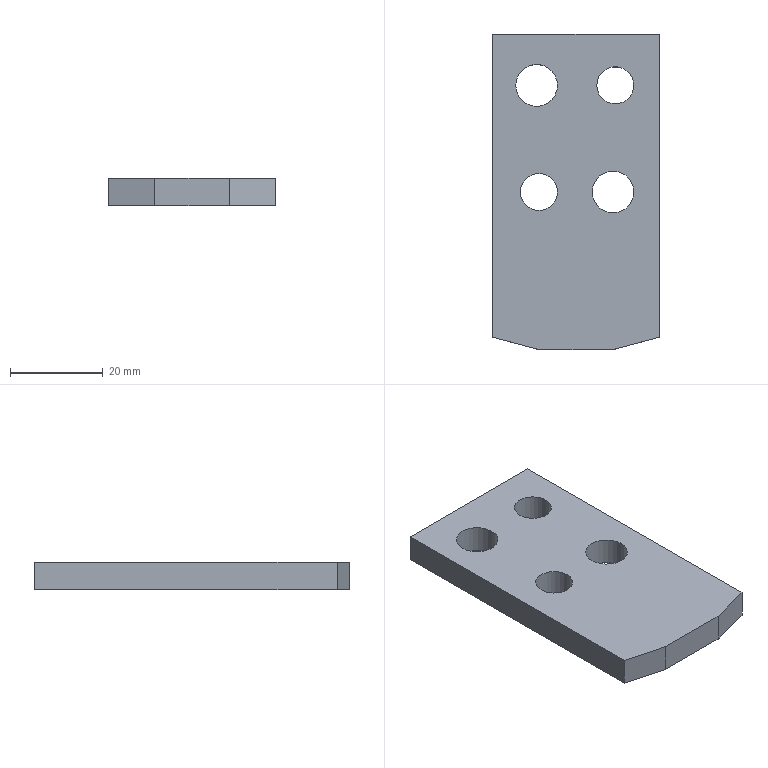Part | STEP file | gslz 2016.10.28-13_id1742_x_t | 1 solid | 12 faces | box 36 x 68 x 6 mm | volume 13161 mm3 | plane 8 | cylinder 4 | commonest cylinder face diameters 8 x2 9 x2
STEP:
#1=CARTESIAN_POINT('',(0.,0.,0.));
#2=DIRECTION('',(0.,0.,1.));
#3=DIRECTION('',(1.,0.,0.));
#4=AXIS2_PLACEMENT_3D('',#1,#2,#3);
#5=CARTESIAN_POINT('',(-870.002,304.2,6.));
#6=VERTEX_POINT('',#5);
#7=CARTESIAN_POINT('',(-878.002,304.2,6.));
#8=VERTEX_POINT('',#7);
#9=CARTESIAN_POINT('',(-874.002,304.2,6.));
#10=DIRECTION('',(0.,0.,1.));
#11=DIRECTION('',(-1.,0.,0.));
#12=AXIS2_PLACEMENT_3D('',#9,#10,#11);
#13=CIRCLE('',#12,4.);
#14=CARTESIAN_POINT('',(-874.002,304.2,-73.));
#15=DIRECTION('',(0.,0.,1.));
#16=DIRECTION('',(1.,0.,0.));
#17=AXIS2_PLACEMENT_3D('',#14,#15,#16);
#18=CYLINDRICAL_SURFACE('',#17,4.);
#19=CARTESIAN_POINT('',(-3.142,79.));
#20=DIRECTION('',(1.,0.));
#21=VECTOR('',#20,1.);
#22=LINE('',#19,#21);
#23=(GEOMETRIC_REPRESENTATION_CONTEXT(2)PARAMETRIC_REPRESENTATION_CONTEXT()REPRESENTATION_CONTEXT('',''));
#24=DEFINITIONAL_REPRESENTATION('',(#22),#23);
#25=PCURVE('',#18,#24);
#26=CARTESIAN_POINT('',(-941.002,267.7,6.));
#27=DIRECTION('',(0.,0.,-1.));
#28=DIRECTION('',(-1.,0.,0.));
#29=AXIS2_PLACEMENT_3D('',#26,#27,#28);
#30=PLANE('',#29);
#31=CARTESIAN_POINT('',(-63.,36.5));
#32=CARTESIAN_POINT('',(-63.,29.572));
#33=CARTESIAN_POINT('',(-69.,33.036));
#34=CARTESIAN_POINT('',(-75.,36.5));
#35=CARTESIAN_POINT('',(-69.,39.964));
#36=CARTESIAN_POINT('',(-63.,43.428));
#37=CARTESIAN_POINT('',(-63.,36.5));
#38=(BOUNDED_CURVE()B_SPLINE_CURVE(2,(#31,#32,#33,#34,#35,#36,#37),.UNSPECIFIED.,.T.,.F.)B_SPLINE_CURVE_WITH_KNOTS((1,2,2,2,2,1),(-2.094,0.,2.094,4.189,6.283,8.378),.UNSPECIFIED.)CURVE()GEOMETRIC_REPRESENTATION_ITEM()RATIONAL_B_SPLINE_CURVE((1.,0.5,1.,0.5,1.,0.5,1.))REPRESENTATION_ITEM(''));
#39=(GEOMETRIC_REPRESENTATION_CONTEXT(2)PARAMETRIC_REPRESENTATION_CONTEXT()REPRESENTATION_CONTEXT('',''));
#40=DEFINITIONAL_REPRESENTATION('',(#38),#39);
#41=PCURVE('',#30,#40);
#42=SURFACE_CURVE('',#13,(#25,#41),.PCURVE_S1.);
#43=EDGE_CURVE('',#6,#8,#42,.T.);
#44=ORIENTED_EDGE('',*,*,#43,.F.);
#45=CARTESIAN_POINT('',(-870.002,304.2,0.));
#46=VERTEX_POINT('',#45);
#47=CARTESIAN_POINT('',(-870.002,304.2,0.));
#48=CARTESIAN_POINT('',(-870.002,304.2,6.));
#49=B_SPLINE_CURVE_WITH_KNOTS('',1,(#47,#48),.UNSPECIFIED.,.F.,.F.,(2,2),(73.,79.),.PIECEWISE_BEZIER_KNOTS.);
#50=CARTESIAN_POINT('',(0.,0.));
#51=DIRECTION('',(0.,1.));
#52=VECTOR('',#51,1.);
#53=LINE('',#50,#52);
#54=(GEOMETRIC_REPRESENTATION_CONTEXT(2)PARAMETRIC_REPRESENTATION_CONTEXT()REPRESENTATION_CONTEXT('',''));
#55=DEFINITIONAL_REPRESENTATION('',(#53),#54);
#56=PCURVE('',#18,#55);
#57=CARTESIAN_POINT('',(6.283,0.));
#58=DIRECTION('',(0.,1.));
#59=VECTOR('',#58,1.);
#60=LINE('',#57,#59);
#61=(GEOMETRIC_REPRESENTATION_CONTEXT(2)PARAMETRIC_REPRESENTATION_CONTEXT()REPRESENTATION_CONTEXT('',''));
#62=DEFINITIONAL_REPRESENTATION('',(#60),#61);
#63=PCURVE('',#18,#62);
#64=SEAM_CURVE('',#49,(#56,#63),.PCURVE_S1.);
#65=EDGE_CURVE('',#46,#6,#64,.T.);
#66=ORIENTED_EDGE('',*,*,#65,.F.);
#67=CARTESIAN_POINT('',(-874.002,304.2,0.));
#68=DIRECTION('',(0.,0.,-1.));
#69=DIRECTION('',(1.,0.,0.));
#70=AXIS2_PLACEMENT_3D('',#67,#68,#69);
#71=CIRCLE('',#70,4.);
#72=CARTESIAN_POINT('',(6.283,73.));
#73=DIRECTION('',(-1.,0.));
#74=VECTOR('',#73,1.);
#75=LINE('',#72,#74);
#76=(GEOMETRIC_REPRESENTATION_CONTEXT(2)PARAMETRIC_REPRESENTATION_CONTEXT()REPRESENTATION_CONTEXT('',''));
#77=DEFINITIONAL_REPRESENTATION('',(#75),#76);
#78=PCURVE('',#18,#77);
#79=CARTESIAN_POINT('',(-981.002,298.2,0.));
#80=DIRECTION('',(0.,0.,1.));
#81=DIRECTION('',(1.,0.,0.));
#82=AXIS2_PLACEMENT_3D('',#79,#80,#81);
#83=PLANE('',#82);
#84=CARTESIAN_POINT('',(111.,6.));
#85=CARTESIAN_POINT('',(111.,-0.9282));
#86=CARTESIAN_POINT('',(105.,2.536));
#87=CARTESIAN_POINT('',(99.,6.));
#88=CARTESIAN_POINT('',(105.,9.464));
#89=CARTESIAN_POINT('',(111.,12.928));
#90=CARTESIAN_POINT('',(111.,6.));
#91=(BOUNDED_CURVE()B_SPLINE_CURVE(2,(#84,#85,#86,#87,#88,#89,#90),.UNSPECIFIED.,.T.,.F.)B_SPLINE_CURVE_WITH_KNOTS((1,2,2,2,2,1),(-2.094,0.,2.094,4.189,6.283,8.378),.UNSPECIFIED.)CURVE()GEOMETRIC_REPRESENTATION_ITEM()RATIONAL_B_SPLINE_CURVE((1.,0.5,1.,0.5,1.,0.5,1.))REPRESENTATION_ITEM(''));
#92=(GEOMETRIC_REPRESENTATION_CONTEXT(2)PARAMETRIC_REPRESENTATION_CONTEXT()REPRESENTATION_CONTEXT('',''));
#93=DEFINITIONAL_REPRESENTATION('',(#91),#92);
#94=PCURVE('',#83,#93);
#95=SURFACE_CURVE('',#71,(#78,#94),.PCURVE_S1.);
#96=EDGE_CURVE('',#46,#46,#95,.T.);
#97=ORIENTED_EDGE('',*,*,#96,.F.);
#98=ORIENTED_EDGE('',*,*,#65,.T.);
#99=CARTESIAN_POINT('',(-874.002,304.2,6.));
#100=DIRECTION('',(0.,0.,1.));
#101=DIRECTION('',(-1.,0.,0.));
#102=AXIS2_PLACEMENT_3D('',#99,#100,#101);
#103=CIRCLE('',#102,4.);
#104=CARTESIAN_POINT('',(3.142,79.));
#105=DIRECTION('',(1.,0.));
#106=VECTOR('',#105,1.);
#107=LINE('',#104,#106);
#108=(GEOMETRIC_REPRESENTATION_CONTEXT(2)PARAMETRIC_REPRESENTATION_CONTEXT()REPRESENTATION_CONTEXT('',''));
#109=DEFINITIONAL_REPRESENTATION('',(#107),#108);
#110=PCURVE('',#18,#109);
#111=CARTESIAN_POINT('',(-63.,36.5));
#112=CARTESIAN_POINT('',(-63.,29.572));
#113=CARTESIAN_POINT('',(-69.,33.036));
#114=CARTESIAN_POINT('',(-75.,36.5));
#115=CARTESIAN_POINT('',(-69.,39.964));
#116=CARTESIAN_POINT('',(-63.,43.428));
#117=CARTESIAN_POINT('',(-63.,36.5));
#118=(BOUNDED_CURVE()B_SPLINE_CURVE(2,(#111,#112,#113,#114,#115,#116,#117),.UNSPECIFIED.,.T.,.F.)B_SPLINE_CURVE_WITH_KNOTS((1,2,2,2,2,1),(-2.094,0.,2.094,4.189,6.283,8.378),.UNSPECIFIED.)CURVE()GEOMETRIC_REPRESENTATION_ITEM()RATIONAL_B_SPLINE_CURVE((1.,0.5,1.,0.5,1.,0.5,1.))REPRESENTATION_ITEM(''));
#119=(GEOMETRIC_REPRESENTATION_CONTEXT(2)PARAMETRIC_REPRESENTATION_CONTEXT()REPRESENTATION_CONTEXT('',''));
#120=DEFINITIONAL_REPRESENTATION('',(#118),#119);
#121=PCURVE('',#30,#120);
#122=SURFACE_CURVE('',#103,(#110,#121),.PCURVE_S1.);
#123=EDGE_CURVE('',#8,#6,#122,.T.);
#124=ORIENTED_EDGE('',*,*,#123,.F.);
#125=EDGE_LOOP('',(#44,#66,#97,#98,#124));
#126=FACE_BOUND('',#125,.F.);
#127=ADVANCED_FACE('',(#126),#18,.F.);
#128=CARTESIAN_POINT('',(-862.502,304.2,6.));
#129=VERTEX_POINT('',#128);
#130=CARTESIAN_POINT('',(-853.502,304.2,6.));
#131=VERTEX_POINT('',#130);
#132=CARTESIAN_POINT('',(-858.002,304.2,6.));
#133=DIRECTION('',(0.,0.,-1.));
#134=DIRECTION('',(-1.,0.,0.));
#135=AXIS2_PLACEMENT_3D('',#132,#133,#134);
#136=CIRCLE('',#135,4.5);
#137=CARTESIAN_POINT('',(-858.002,304.2,-73.));
#138=DIRECTION('',(0.,0.,1.));
#139=DIRECTION('',(1.,0.,0.));
#140=AXIS2_PLACEMENT_3D('',#137,#138,#139);
#141=CYLINDRICAL_SURFACE('',#140,4.5);
#142=CARTESIAN_POINT('',(3.142,79.));
#143=DIRECTION('',(-1.,0.));
#144=VECTOR('',#143,1.);
#145=LINE('',#142,#144);
#146=(GEOMETRIC_REPRESENTATION_CONTEXT(2)PARAMETRIC_REPRESENTATION_CONTEXT()REPRESENTATION_CONTEXT('',''));
#147=DEFINITIONAL_REPRESENTATION('',(#145),#146);
#148=PCURVE('',#141,#147);
#149=CARTESIAN_POINT('',(-83.,36.5));
#150=DIRECTION('',(1.,0.));
#151=AXIS2_PLACEMENT_2D('',#149,#150);
#152=CIRCLE('',#151,4.5);
#153=(GEOMETRIC_REPRESENTATION_CONTEXT(2)PARAMETRIC_REPRESENTATION_CONTEXT()REPRESENTATION_CONTEXT('',''));
#154=DEFINITIONAL_REPRESENTATION('',(#152),#153);
#155=PCURVE('',#30,#154);
#156=SURFACE_CURVE('',#136,(#148,#155),.PCURVE_S1.);
#157=EDGE_CURVE('',#129,#131,#156,.T.);
#158=ORIENTED_EDGE('',*,*,#157,.T.);
#159=CARTESIAN_POINT('',(-853.502,304.2,0.));
#160=VERTEX_POINT('',#159);
#161=CARTESIAN_POINT('',(-853.502,304.2,0.));
#162=CARTESIAN_POINT('',(-853.502,304.2,6.));
#163=B_SPLINE_CURVE_WITH_KNOTS('',1,(#161,#162),.UNSPECIFIED.,.F.,.F.,(2,2),(73.,79.),.PIECEWISE_BEZIER_KNOTS.);
#164=CARTESIAN_POINT('',(0.,0.));
#165=DIRECTION('',(0.,1.));
#166=VECTOR('',#165,1.);
#167=LINE('',#164,#166);
#168=(GEOMETRIC_REPRESENTATION_CONTEXT(2)PARAMETRIC_REPRESENTATION_CONTEXT()REPRESENTATION_CONTEXT('',''));
#169=DEFINITIONAL_REPRESENTATION('',(#167),#168);
#170=PCURVE('',#141,#169);
#171=CARTESIAN_POINT('',(6.283,0.));
#172=DIRECTION('',(0.,1.));
#173=VECTOR('',#172,1.);
#174=LINE('',#171,#173);
#175=(GEOMETRIC_REPRESENTATION_CONTEXT(2)PARAMETRIC_REPRESENTATION_CONTEXT()REPRESENTATION_CONTEXT('',''));
#176=DEFINITIONAL_REPRESENTATION('',(#174),#175);
#177=PCURVE('',#141,#176);
#178=SEAM_CURVE('',#163,(#170,#177),.PCURVE_S1.);
#179=EDGE_CURVE('',#160,#131,#178,.T.);
#180=ORIENTED_EDGE('',*,*,#179,.F.);
#181=CARTESIAN_POINT('',(-858.002,304.2,0.));
#182=DIRECTION('',(0.,0.,1.));
#183=DIRECTION('',(1.,0.,0.));
#184=AXIS2_PLACEMENT_3D('',#181,#182,#183);
#185=CIRCLE('',#184,4.5);
#186=CARTESIAN_POINT('',(0.,73.));
#187=DIRECTION('',(1.,0.));
#188=VECTOR('',#187,1.);
#189=LINE('',#186,#188);
#190=(GEOMETRIC_REPRESENTATION_CONTEXT(2)PARAMETRIC_REPRESENTATION_CONTEXT()REPRESENTATION_CONTEXT('',''));
#191=DEFINITIONAL_REPRESENTATION('',(#189),#190);
#192=PCURVE('',#141,#191);
#193=CARTESIAN_POINT('',(123.,6.));
#194=DIRECTION('',(1.,0.));
#195=AXIS2_PLACEMENT_2D('',#193,#194);
#196=CIRCLE('',#195,4.5);
#197=(GEOMETRIC_REPRESENTATION_CONTEXT(2)PARAMETRIC_REPRESENTATION_CONTEXT()REPRESENTATION_CONTEXT('',''));
#198=DEFINITIONAL_REPRESENTATION('',(#196),#197);
#199=PCURVE('',#83,#198);
#200=SURFACE_CURVE('',#185,(#192,#199),.PCURVE_S1.);
#201=EDGE_CURVE('',#160,#160,#200,.T.);
#202=ORIENTED_EDGE('',*,*,#201,.T.);
#203=ORIENTED_EDGE('',*,*,#179,.T.);
#204=CARTESIAN_POINT('',(-858.002,304.2,6.));
#205=DIRECTION('',(0.,0.,-1.));
#206=DIRECTION('',(-1.,0.,0.));
#207=AXIS2_PLACEMENT_3D('',#204,#205,#206);
#208=CIRCLE('',#207,4.5);
#209=CARTESIAN_POINT('',(9.425,79.));
#210=DIRECTION('',(-1.,0.));
#211=VECTOR('',#210,1.);
#212=LINE('',#209,#211);
#213=(GEOMETRIC_REPRESENTATION_CONTEXT(2)PARAMETRIC_REPRESENTATION_CONTEXT()REPRESENTATION_CONTEXT('',''));
#214=DEFINITIONAL_REPRESENTATION('',(#212),#213);
#215=PCURVE('',#141,#214);
#216=CARTESIAN_POINT('',(-83.,36.5));
#217=DIRECTION('',(1.,0.));
#218=AXIS2_PLACEMENT_2D('',#216,#217);
#219=CIRCLE('',#218,4.5);
#220=(GEOMETRIC_REPRESENTATION_CONTEXT(2)PARAMETRIC_REPRESENTATION_CONTEXT()REPRESENTATION_CONTEXT('',''));
#221=DEFINITIONAL_REPRESENTATION('',(#219),#220);
#222=PCURVE('',#30,#221);
#223=SURFACE_CURVE('',#208,(#215,#222),.PCURVE_S1.);
#224=EDGE_CURVE('',#131,#129,#223,.T.);
#225=ORIENTED_EDGE('',*,*,#224,.T.);
#226=EDGE_LOOP('',(#158,#180,#202,#203,#225));
#227=FACE_BOUND('',#226,.F.);
#228=ADVANCED_FACE('',(#227),#141,.F.);
#229=CARTESIAN_POINT('',(-879.002,327.2,6.));
#230=VERTEX_POINT('',#229);
#231=CARTESIAN_POINT('',(-874.502,327.2,6.));
#232=DIRECTION('',(0.,0.,-1.));
#233=DIRECTION('',(-1.,0.,0.));
#234=AXIS2_PLACEMENT_3D('',#231,#232,#233);
#235=CIRCLE('',#234,4.5);
#236=CARTESIAN_POINT('',(-874.502,327.2,47.));
#237=DIRECTION('',(0.,0.,-1.));
#238=DIRECTION('',(-1.,0.,0.));
#239=AXIS2_PLACEMENT_3D('',#236,#237,#238);
#240=CYLINDRICAL_SURFACE('',#239,4.5);
#241=CARTESIAN_POINT('',(0.,41.));
#242=DIRECTION('',(1.,0.));
#243=VECTOR('',#242,1.);
#244=LINE('',#241,#243);
#245=(GEOMETRIC_REPRESENTATION_CONTEXT(2)PARAMETRIC_REPRESENTATION_CONTEXT()REPRESENTATION_CONTEXT('',''));
#246=DEFINITIONAL_REPRESENTATION('',(#244),#245);
#247=PCURVE('',#240,#246);
#248=CARTESIAN_POINT('',(-66.5,59.5));
#249=DIRECTION('',(1.,0.));
#250=AXIS2_PLACEMENT_2D('',#248,#249);
#251=CIRCLE('',#250,4.5);
#252=(GEOMETRIC_REPRESENTATION_CONTEXT(2)PARAMETRIC_REPRESENTATION_CONTEXT()REPRESENTATION_CONTEXT('',''));
#253=DEFINITIONAL_REPRESENTATION('',(#251),#252);
#254=PCURVE('',#30,#253);
#255=SURFACE_CURVE('',#235,(#247,#254),.PCURVE_S1.);
#256=EDGE_CURVE('',#230,#230,#255,.T.);
#257=ORIENTED_EDGE('',*,*,#256,.T.);
#258=CARTESIAN_POINT('',(-879.002,327.2,0.));
#259=VERTEX_POINT('',#258);
#260=CARTESIAN_POINT('',(-879.002,327.2,6.));
#261=CARTESIAN_POINT('',(-879.002,327.2,0.));
#262=B_SPLINE_CURVE_WITH_KNOTS('',1,(#260,#261),.UNSPECIFIED.,.F.,.F.,(2,2),(41.,47.),.PIECEWISE_BEZIER_KNOTS.);
#263=CARTESIAN_POINT('',(6.283,0.));
#264=DIRECTION('',(0.,1.));
#265=VECTOR('',#264,1.);
#266=LINE('',#263,#265);
#267=(GEOMETRIC_REPRESENTATION_CONTEXT(2)PARAMETRIC_REPRESENTATION_CONTEXT()REPRESENTATION_CONTEXT('',''));
#268=DEFINITIONAL_REPRESENTATION('',(#266),#267);
#269=PCURVE('',#240,#268);
#270=CARTESIAN_POINT('',(0.,0.));
#271=DIRECTION('',(0.,1.));
#272=VECTOR('',#271,1.);
#273=LINE('',#270,#272);
#274=(GEOMETRIC_REPRESENTATION_CONTEXT(2)PARAMETRIC_REPRESENTATION_CONTEXT()REPRESENTATION_CONTEXT('',''));
#275=DEFINITIONAL_REPRESENTATION('',(#273),#274);
#276=PCURVE('',#240,#275);
#277=SEAM_CURVE('',#262,(#269,#276),.PCURVE_S1.);
#278=EDGE_CURVE('',#230,#259,#277,.T.);
#279=ORIENTED_EDGE('',*,*,#278,.T.);
#280=CARTESIAN_POINT('',(-870.002,327.2,0.));
#281=VERTEX_POINT('',#280);
#282=CARTESIAN_POINT('',(-874.502,327.2,0.));
#283=DIRECTION('',(0.,0.,1.));
#284=DIRECTION('',(1.,0.,0.));
#285=AXIS2_PLACEMENT_3D('',#282,#283,#284);
#286=CIRCLE('',#285,4.5);
#287=CARTESIAN_POINT('',(9.425,47.));
#288=DIRECTION('',(-1.,0.));
#289=VECTOR('',#288,1.);
#290=LINE('',#287,#289);
#291=(GEOMETRIC_REPRESENTATION_CONTEXT(2)PARAMETRIC_REPRESENTATION_CONTEXT()REPRESENTATION_CONTEXT('',''));
#292=DEFINITIONAL_REPRESENTATION('',(#290),#291);
#293=PCURVE('',#240,#292);
#294=CARTESIAN_POINT('',(106.5,29.));
#295=DIRECTION('',(1.,0.));
#296=AXIS2_PLACEMENT_2D('',#294,#295);
#297=CIRCLE('',#296,4.5);
#298=(GEOMETRIC_REPRESENTATION_CONTEXT(2)PARAMETRIC_REPRESENTATION_CONTEXT()REPRESENTATION_CONTEXT('',''));
#299=DEFINITIONAL_REPRESENTATION('',(#297),#298);
#300=PCURVE('',#83,#299);
#301=SURFACE_CURVE('',#286,(#293,#300),.PCURVE_S1.);
#302=EDGE_CURVE('',#259,#281,#301,.T.);
#303=ORIENTED_EDGE('',*,*,#302,.T.);
#304=CARTESIAN_POINT('',(-874.502,327.2,0.));
#305=DIRECTION('',(0.,0.,1.));
#306=DIRECTION('',(1.,0.,0.));
#307=AXIS2_PLACEMENT_3D('',#304,#305,#306);
#308=CIRCLE('',#307,4.5);
#309=CARTESIAN_POINT('',(3.142,47.));
#310=DIRECTION('',(-1.,0.));
#311=VECTOR('',#310,1.);
#312=LINE('',#309,#311);
#313=(GEOMETRIC_REPRESENTATION_CONTEXT(2)PARAMETRIC_REPRESENTATION_CONTEXT()REPRESENTATION_CONTEXT('',''));
#314=DEFINITIONAL_REPRESENTATION('',(#312),#313);
#315=PCURVE('',#240,#314);
#316=CARTESIAN_POINT('',(106.5,29.));
#317=DIRECTION('',(1.,0.));
#318=AXIS2_PLACEMENT_2D('',#316,#317);
#319=CIRCLE('',#318,4.5);
#320=(GEOMETRIC_REPRESENTATION_CONTEXT(2)PARAMETRIC_REPRESENTATION_CONTEXT()REPRESENTATION_CONTEXT('',''));
#321=DEFINITIONAL_REPRESENTATION('',(#319),#320);
#322=PCURVE('',#83,#321);
#323=SURFACE_CURVE('',#308,(#315,#322),.PCURVE_S1.);
#324=EDGE_CURVE('',#281,#259,#323,.T.);
#325=ORIENTED_EDGE('',*,*,#324,.T.);
#326=ORIENTED_EDGE('',*,*,#278,.F.);
#327=EDGE_LOOP('',(#257,#279,#303,#325,#326));
#328=FACE_BOUND('',#327,.F.);
#329=ADVANCED_FACE('',(#328),#240,.F.);
#330=CARTESIAN_POINT('',(-858.001,270.2,0.));
#331=VERTEX_POINT('',#330);
#332=CARTESIAN_POINT('',(-858.001,270.2,6.));
#333=VERTEX_POINT('',#332);
#334=CARTESIAN_POINT('',(-858.001,270.2,8.));
#335=DIRECTION('',(0.,0.,1.));
#336=VECTOR('',#335,1.);
#337=LINE('',#334,#336);
#338=CARTESIAN_POINT('',(-971.,270.2,8.));
#339=DIRECTION('',(0.,1.,0.));
#340=DIRECTION('',(0.,0.,1.));
#341=AXIS2_PLACEMENT_3D('',#338,#339,#340);
#342=PLANE('',#341);
#343=CARTESIAN_POINT('',(0.,112.999));
#344=DIRECTION('',(1.,0.));
#345=VECTOR('',#344,1.);
#346=LINE('',#343,#345);
#347=(GEOMETRIC_REPRESENTATION_CONTEXT(2)PARAMETRIC_REPRESENTATION_CONTEXT()REPRESENTATION_CONTEXT('',''));
#348=DEFINITIONAL_REPRESENTATION('',(#346),#347);
#349=PCURVE('',#342,#348);
#350=CARTESIAN_POINT('',(-858.001,270.2,8.));
#351=DIRECTION('',(-0.2588,0.9659,0.));
#352=DIRECTION('',(-0.9659,-0.2588,0.));
#353=AXIS2_PLACEMENT_3D('',#350,#351,#352);
#354=PLANE('',#353);
#355=CARTESIAN_POINT('',(0.,0.));
#356=DIRECTION('',(0.,1.));
#357=VECTOR('',#356,1.);
#358=LINE('',#355,#357);
#359=(GEOMETRIC_REPRESENTATION_CONTEXT(2)PARAMETRIC_REPRESENTATION_CONTEXT()REPRESENTATION_CONTEXT('',''));
#360=DEFINITIONAL_REPRESENTATION('',(#358),#359);
#361=PCURVE('',#354,#360);
#362=SURFACE_CURVE('',#337,(#349,#361),.PCURVE_S1.);
#363=EDGE_CURVE('',#331,#333,#362,.T.);
#364=ORIENTED_EDGE('',*,*,#363,.T.);
#365=CARTESIAN_POINT('',(-874.,270.2,6.));
#366=VERTEX_POINT('',#365);
#367=CARTESIAN_POINT('',(-971.,270.2,6.));
#368=DIRECTION('',(-1.,0.,0.));
#369=VECTOR('',#368,1.);
#370=LINE('',#367,#369);
#371=CARTESIAN_POINT('',(-2.,0.));
#372=DIRECTION('',(0.,-1.));
#373=VECTOR('',#372,1.);
#374=LINE('',#371,#373);
#375=(GEOMETRIC_REPRESENTATION_CONTEXT(2)PARAMETRIC_REPRESENTATION_CONTEXT()REPRESENTATION_CONTEXT('',''));
#376=DEFINITIONAL_REPRESENTATION('',(#374),#375);
#377=PCURVE('',#342,#376);
#378=CARTESIAN_POINT('',(29.998,2.5));
#379=DIRECTION('',(1.,0.));
#380=VECTOR('',#379,1.);
#381=LINE('',#378,#380);
#382=(GEOMETRIC_REPRESENTATION_CONTEXT(2)PARAMETRIC_REPRESENTATION_CONTEXT()REPRESENTATION_CONTEXT('',''));
#383=DEFINITIONAL_REPRESENTATION('',(#381),#382);
#384=PCURVE('',#30,#383);
#385=SURFACE_CURVE('',#370,(#377,#384),.PCURVE_S1.);
#386=EDGE_CURVE('',#333,#366,#385,.T.);
#387=ORIENTED_EDGE('',*,*,#386,.T.);
#388=CARTESIAN_POINT('',(-874.,270.2,0.));
#389=VERTEX_POINT('',#388);
#390=CARTESIAN_POINT('',(-874.,270.2,8.));
#391=DIRECTION('',(0.,0.,1.));
#392=VECTOR('',#391,1.);
#393=LINE('',#390,#392);
#394=CARTESIAN_POINT('',(0.,97.));
#395=DIRECTION('',(1.,0.));
#396=VECTOR('',#395,1.);
#397=LINE('',#394,#396);
#398=(GEOMETRIC_REPRESENTATION_CONTEXT(2)PARAMETRIC_REPRESENTATION_CONTEXT()REPRESENTATION_CONTEXT('',''));
#399=DEFINITIONAL_REPRESENTATION('',(#397),#398);
#400=PCURVE('',#342,#399);
#401=CARTESIAN_POINT('',(-884.002,272.88,8.));
#402=DIRECTION('',(0.2588,0.9659,0.));
#403=DIRECTION('',(-0.9659,0.2588,0.));
#404=AXIS2_PLACEMENT_3D('',#401,#402,#403);
#405=PLANE('',#404);
#406=CARTESIAN_POINT('',(-10.355,0.));
#407=DIRECTION('',(0.,1.));
#408=VECTOR('',#407,1.);
#409=LINE('',#406,#408);
#410=(GEOMETRIC_REPRESENTATION_CONTEXT(2)PARAMETRIC_REPRESENTATION_CONTEXT()REPRESENTATION_CONTEXT('',''));
#411=DEFINITIONAL_REPRESENTATION('',(#409),#410);
#412=PCURVE('',#405,#411);
#413=SURFACE_CURVE('',#393,(#400,#412),.PCURVE_S1.);
#414=EDGE_CURVE('',#389,#366,#413,.T.);
#415=ORIENTED_EDGE('',*,*,#414,.F.);
#416=CARTESIAN_POINT('',(-971.,270.2,0.));
#417=DIRECTION('',(1.,0.,0.));
#418=VECTOR('',#417,1.);
#419=LINE('',#416,#418);
#420=CARTESIAN_POINT('',(-8.,0.));
#421=DIRECTION('',(0.,1.));
#422=VECTOR('',#421,1.);
#423=LINE('',#420,#422);
#424=(GEOMETRIC_REPRESENTATION_CONTEXT(2)PARAMETRIC_REPRESENTATION_CONTEXT()REPRESENTATION_CONTEXT('',''));
#425=DEFINITIONAL_REPRESENTATION('',(#423),#424);
#426=PCURVE('',#342,#425);
#427=CARTESIAN_POINT('',(10.002,-28.));
#428=DIRECTION('',(1.,0.));
#429=VECTOR('',#428,1.);
#430=LINE('',#427,#429);
#431=(GEOMETRIC_REPRESENTATION_CONTEXT(2)PARAMETRIC_REPRESENTATION_CONTEXT()REPRESENTATION_CONTEXT('',''));
#432=DEFINITIONAL_REPRESENTATION('',(#430),#431);
#433=PCURVE('',#83,#432);
#434=SURFACE_CURVE('',#419,(#426,#433),.PCURVE_S1.);
#435=EDGE_CURVE('',#389,#331,#434,.T.);
#436=ORIENTED_EDGE('',*,*,#435,.T.);
#437=EDGE_LOOP('',(#364,#387,#415,#436));
#438=FACE_BOUND('',#437,.T.);
#439=ADVANCED_FACE('',(#438),#342,.F.);
#440=CARTESIAN_POINT('',(-848.002,272.879,6.));
#441=VERTEX_POINT('',#440);
#442=CARTESIAN_POINT('',(-848.002,272.879,0.));
#443=VERTEX_POINT('',#442);
#444=CARTESIAN_POINT('',(-848.002,272.879,8.));
#445=DIRECTION('',(0.,0.,-1.));
#446=VECTOR('',#445,1.);
#447=LINE('',#444,#446);
#448=CARTESIAN_POINT('',(-10.352,0.));
#449=DIRECTION('',(0.,-1.));
#450=VECTOR('',#449,1.);
#451=LINE('',#448,#450);
#452=(GEOMETRIC_REPRESENTATION_CONTEXT(2)PARAMETRIC_REPRESENTATION_CONTEXT()REPRESENTATION_CONTEXT('',''));
#453=DEFINITIONAL_REPRESENTATION('',(#451),#452);
#454=PCURVE('',#354,#453);
#455=CARTESIAN_POINT('',(-848.002,265.2,16.));
#456=DIRECTION('',(-1.,0.,0.));
#457=DIRECTION('',(0.,0.,1.));
#458=AXIS2_PLACEMENT_3D('',#455,#456,#457);
#459=PLANE('',#458);
#460=CARTESIAN_POINT('',(-8.,7.679));
#461=DIRECTION('',(-1.,0.));
#462=VECTOR('',#461,1.);
#463=LINE('',#460,#462);
#464=(GEOMETRIC_REPRESENTATION_CONTEXT(2)PARAMETRIC_REPRESENTATION_CONTEXT()REPRESENTATION_CONTEXT('',''));
#465=DEFINITIONAL_REPRESENTATION('',(#463),#464);
#466=PCURVE('',#459,#465);
#467=SURFACE_CURVE('',#447,(#454,#466),.PCURVE_S1.);
#468=EDGE_CURVE('',#441,#443,#467,.T.);
#469=ORIENTED_EDGE('',*,*,#468,.F.);
#470=CARTESIAN_POINT('',(-858.001,270.2,6.));
#471=DIRECTION('',(-0.9659,-0.2588,0.));
#472=VECTOR('',#471,1.);
#473=LINE('',#470,#472);
#474=CARTESIAN_POINT('',(0.,-2.));
#475=DIRECTION('',(1.,0.));
#476=VECTOR('',#475,1.);
#477=LINE('',#474,#476);
#478=(GEOMETRIC_REPRESENTATION_CONTEXT(2)PARAMETRIC_REPRESENTATION_CONTEXT()REPRESENTATION_CONTEXT('',''));
#479=DEFINITIONAL_REPRESENTATION('',(#477),#478);
#480=PCURVE('',#354,#479);
#481=CARTESIAN_POINT('',(-83.001,2.5));
#482=DIRECTION('',(0.9659,-0.2588));
#483=VECTOR('',#482,1.);
#484=LINE('',#481,#483);
#485=(GEOMETRIC_REPRESENTATION_CONTEXT(2)PARAMETRIC_REPRESENTATION_CONTEXT()REPRESENTATION_CONTEXT('',''));
#486=DEFINITIONAL_REPRESENTATION('',(#484),#485);
#487=PCURVE('',#30,#486);
#488=SURFACE_CURVE('',#473,(#480,#487),.PCURVE_S1.);
#489=EDGE_CURVE('',#441,#333,#488,.T.);
#490=ORIENTED_EDGE('',*,*,#489,.T.);
#491=ORIENTED_EDGE('',*,*,#363,.F.);
#492=CARTESIAN_POINT('',(-858.001,270.2,0.));
#493=DIRECTION('',(0.9659,0.2588,0.));
#494=VECTOR('',#493,1.);
#495=LINE('',#492,#494);
#496=CARTESIAN_POINT('',(0.,-8.));
#497=DIRECTION('',(-1.,0.));
#498=VECTOR('',#497,1.);
#499=LINE('',#496,#498);
#500=(GEOMETRIC_REPRESENTATION_CONTEXT(2)PARAMETRIC_REPRESENTATION_CONTEXT()REPRESENTATION_CONTEXT('',''));
#501=DEFINITIONAL_REPRESENTATION('',(#499),#500);
#502=PCURVE('',#354,#501);
#503=CARTESIAN_POINT('',(123.001,-28.));
#504=DIRECTION('',(0.9659,0.2588));
#505=VECTOR('',#504,1.);
#506=LINE('',#503,#505);
#507=(GEOMETRIC_REPRESENTATION_CONTEXT(2)PARAMETRIC_REPRESENTATION_CONTEXT()REPRESENTATION_CONTEXT('',''));
#508=DEFINITIONAL_REPRESENTATION('',(#506),#507);
#509=PCURVE('',#83,#508);
#510=SURFACE_CURVE('',#495,(#502,#509),.PCURVE_S1.);
#511=EDGE_CURVE('',#331,#443,#510,.T.);
#512=ORIENTED_EDGE('',*,*,#511,.T.);
#513=EDGE_LOOP('',(#469,#490,#491,#512));
#514=FACE_BOUND('',#513,.T.);
#515=ADVANCED_FACE('',(#514),#354,.F.);
#516=CARTESIAN_POINT('',(-848.002,338.2,6.));
#517=VERTEX_POINT('',#516);
#518=CARTESIAN_POINT('',(-848.002,338.2,0.));
#519=VERTEX_POINT('',#518);
#520=CARTESIAN_POINT('',(-848.002,338.2,16.));
#521=DIRECTION('',(0.,0.,-1.));
#522=VECTOR('',#521,1.);
#523=LINE('',#520,#522);
#524=CARTESIAN_POINT('',(0.,73.));
#525=DIRECTION('',(-1.,0.));
#526=VECTOR('',#525,1.);
#527=LINE('',#524,#526);
#528=(GEOMETRIC_REPRESENTATION_CONTEXT(2)PARAMETRIC_REPRESENTATION_CONTEXT()REPRESENTATION_CONTEXT('',''));
#529=DEFINITIONAL_REPRESENTATION('',(#527),#528);
#530=PCURVE('',#459,#529);
#531=CARTESIAN_POINT('',(-901.002,338.2,16.));
#532=DIRECTION('',(0.,-1.,0.));
#533=DIRECTION('',(0.,0.,-1.));
#534=AXIS2_PLACEMENT_3D('',#531,#532,#533);
#535=PLANE('',#534);
#536=CARTESIAN_POINT('',(0.,53.));
#537=DIRECTION('',(1.,0.));
#538=VECTOR('',#537,1.);
#539=LINE('',#536,#538);
#540=(GEOMETRIC_REPRESENTATION_CONTEXT(2)PARAMETRIC_REPRESENTATION_CONTEXT()REPRESENTATION_CONTEXT('',''));
#541=DEFINITIONAL_REPRESENTATION('',(#539),#540);
#542=PCURVE('',#535,#541);
#543=SURFACE_CURVE('',#523,(#530,#542),.PCURVE_S1.);
#544=EDGE_CURVE('',#517,#519,#543,.T.);
#545=ORIENTED_EDGE('',*,*,#544,.F.);
#546=CARTESIAN_POINT('',(-848.002,265.2,6.));
#547=DIRECTION('',(0.,-1.,0.));
#548=VECTOR('',#547,1.);
#549=LINE('',#546,#548);
#550=CARTESIAN_POINT('',(-10.,0.));
#551=DIRECTION('',(0.,-1.));
#552=VECTOR('',#551,1.);
#553=LINE('',#550,#552);
#554=(GEOMETRIC_REPRESENTATION_CONTEXT(2)PARAMETRIC_REPRESENTATION_CONTEXT()REPRESENTATION_CONTEXT('',''));
#555=DEFINITIONAL_REPRESENTATION('',(#553),#554);
#556=PCURVE('',#459,#555);
#557=CARTESIAN_POINT('',(-93.,-2.5));
#558=DIRECTION('',(0.,-1.));
#559=VECTOR('',#558,1.);
#560=LINE('',#557,#559);
#561=(GEOMETRIC_REPRESENTATION_CONTEXT(2)PARAMETRIC_REPRESENTATION_CONTEXT()REPRESENTATION_CONTEXT('',''));
#562=DEFINITIONAL_REPRESENTATION('',(#560),#561);
#563=PCURVE('',#30,#562);
#564=SURFACE_CURVE('',#549,(#556,#563),.PCURVE_S1.);
#565=EDGE_CURVE('',#517,#441,#564,.T.);
#566=ORIENTED_EDGE('',*,*,#565,.T.);
#567=ORIENTED_EDGE('',*,*,#468,.T.);
#568=CARTESIAN_POINT('',(-848.002,265.2,0.));
#569=DIRECTION('',(0.,1.,0.));
#570=VECTOR('',#569,1.);
#571=LINE('',#568,#570);
#572=CARTESIAN_POINT('',(-16.,0.));
#573=DIRECTION('',(0.,1.));
#574=VECTOR('',#573,1.);
#575=LINE('',#572,#574);
#576=(GEOMETRIC_REPRESENTATION_CONTEXT(2)PARAMETRIC_REPRESENTATION_CONTEXT()REPRESENTATION_CONTEXT('',''));
#577=DEFINITIONAL_REPRESENTATION('',(#575),#576);
#578=PCURVE('',#459,#577);
#579=CARTESIAN_POINT('',(133.,-33.));
#580=DIRECTION('',(0.,1.));
#581=VECTOR('',#580,1.);
#582=LINE('',#579,#581);
#583=(GEOMETRIC_REPRESENTATION_CONTEXT(2)PARAMETRIC_REPRESENTATION_CONTEXT()REPRESENTATION_CONTEXT('',''));
#584=DEFINITIONAL_REPRESENTATION('',(#582),#583);
#585=PCURVE('',#83,#584);
#586=SURFACE_CURVE('',#571,(#578,#585),.PCURVE_S1.);
#587=EDGE_CURVE('',#443,#519,#586,.T.);
#588=ORIENTED_EDGE('',*,*,#587,.T.);
#589=EDGE_LOOP('',(#545,#566,#567,#588));
#590=FACE_BOUND('',#589,.T.);
#591=ADVANCED_FACE('',(#590),#459,.F.);
#592=CARTESIAN_POINT('',(-884.002,338.2,6.));
#593=VERTEX_POINT('',#592);
#594=CARTESIAN_POINT('',(-884.002,338.2,0.));
#595=VERTEX_POINT('',#594);
#596=CARTESIAN_POINT('',(-884.002,338.2,16.));
#597=DIRECTION('',(0.,0.,-1.));
#598=VECTOR('',#597,1.);
#599=LINE('',#596,#598);
#600=CARTESIAN_POINT('',(0.,17.));
#601=DIRECTION('',(1.,0.));
#602=VECTOR('',#601,1.);
#603=LINE('',#600,#602);
#604=(GEOMETRIC_REPRESENTATION_CONTEXT(2)PARAMETRIC_REPRESENTATION_CONTEXT()REPRESENTATION_CONTEXT('',''));
#605=DEFINITIONAL_REPRESENTATION('',(#603),#604);
#606=PCURVE('',#535,#605);
#607=CARTESIAN_POINT('',(-884.002,298.2,16.));
#608=DIRECTION('',(1.,0.,0.));
#609=DIRECTION('',(0.,0.,-1.));
#610=AXIS2_PLACEMENT_3D('',#607,#608,#609);
#611=PLANE('',#610);
#612=CARTESIAN_POINT('',(0.,40.));
#613=DIRECTION('',(1.,0.));
#614=VECTOR('',#613,1.);
#615=LINE('',#612,#614);
#616=(GEOMETRIC_REPRESENTATION_CONTEXT(2)PARAMETRIC_REPRESENTATION_CONTEXT()REPRESENTATION_CONTEXT('',''));
#617=DEFINITIONAL_REPRESENTATION('',(#615),#616);
#618=PCURVE('',#611,#617);
#619=SURFACE_CURVE('',#599,(#606,#618),.PCURVE_S1.);
#620=EDGE_CURVE('',#593,#595,#619,.T.);
#621=ORIENTED_EDGE('',*,*,#620,.F.);
#622=CARTESIAN_POINT('',(-901.002,338.2,6.));
#623=DIRECTION('',(1.,0.,0.));
#624=VECTOR('',#623,1.);
#625=LINE('',#622,#624);
#626=CARTESIAN_POINT('',(10.,0.));
#627=DIRECTION('',(0.,1.));
#628=VECTOR('',#627,1.);
#629=LINE('',#626,#628);
#630=(GEOMETRIC_REPRESENTATION_CONTEXT(2)PARAMETRIC_REPRESENTATION_CONTEXT()REPRESENTATION_CONTEXT('',''));
#631=DEFINITIONAL_REPRESENTATION('',(#629),#630);
#632=PCURVE('',#535,#631);
#633=CARTESIAN_POINT('',(-40.,70.5));
#634=DIRECTION('',(-1.,0.));
#635=VECTOR('',#634,1.);
#636=LINE('',#633,#635);
#637=(GEOMETRIC_REPRESENTATION_CONTEXT(2)PARAMETRIC_REPRESENTATION_CONTEXT()REPRESENTATION_CONTEXT('',''));
#638=DEFINITIONAL_REPRESENTATION('',(#636),#637);
#639=PCURVE('',#30,#638);
#640=SURFACE_CURVE('',#625,(#632,#639),.PCURVE_S1.);
#641=EDGE_CURVE('',#593,#517,#640,.T.);
#642=ORIENTED_EDGE('',*,*,#641,.T.);
#643=ORIENTED_EDGE('',*,*,#544,.T.);
#644=CARTESIAN_POINT('',(-901.002,338.2,0.));
#645=DIRECTION('',(-1.,0.,0.));
#646=VECTOR('',#645,1.);
#647=LINE('',#644,#646);
#648=CARTESIAN_POINT('',(16.,0.));
#649=DIRECTION('',(0.,-1.));
#650=VECTOR('',#649,1.);
#651=LINE('',#648,#650);
#652=(GEOMETRIC_REPRESENTATION_CONTEXT(2)PARAMETRIC_REPRESENTATION_CONTEXT()REPRESENTATION_CONTEXT('',''));
#653=DEFINITIONAL_REPRESENTATION('',(#651),#652);
#654=PCURVE('',#535,#653);
#655=CARTESIAN_POINT('',(80.,40.));
#656=DIRECTION('',(-1.,0.));
#657=VECTOR('',#656,1.);
#658=LINE('',#655,#657);
#659=(GEOMETRIC_REPRESENTATION_CONTEXT(2)PARAMETRIC_REPRESENTATION_CONTEXT()REPRESENTATION_CONTEXT('',''));
#660=DEFINITIONAL_REPRESENTATION('',(#658),#659);
#661=PCURVE('',#83,#660);
#662=SURFACE_CURVE('',#647,(#654,#661),.PCURVE_S1.);
#663=EDGE_CURVE('',#519,#595,#662,.T.);
#664=ORIENTED_EDGE('',*,*,#663,.T.);
#665=EDGE_LOOP('',(#621,#642,#643,#664));
#666=FACE_BOUND('',#665,.T.);
#667=ADVANCED_FACE('',(#666),#535,.F.);
#668=CARTESIAN_POINT('',(-884.002,272.88,6.));
#669=VERTEX_POINT('',#668);
#670=CARTESIAN_POINT('',(-884.002,272.88,0.));
#671=VERTEX_POINT('',#670);
#672=CARTESIAN_POINT('',(-884.002,272.88,8.));
#673=DIRECTION('',(0.,0.,-1.));
#674=VECTOR('',#673,1.);
#675=LINE('',#672,#674);
#676=CARTESIAN_POINT('',(8.,-25.32));
#677=DIRECTION('',(1.,0.));
#678=VECTOR('',#677,1.);
#679=LINE('',#676,#678);
#680=(GEOMETRIC_REPRESENTATION_CONTEXT(2)PARAMETRIC_REPRESENTATION_CONTEXT()REPRESENTATION_CONTEXT('',''));
#681=DEFINITIONAL_REPRESENTATION('',(#679),#680);
#682=PCURVE('',#611,#681);
#683=CARTESIAN_POINT('',(0.,0.));
#684=DIRECTION('',(0.,-1.));
#685=VECTOR('',#684,1.);
#686=LINE('',#683,#685);
#687=(GEOMETRIC_REPRESENTATION_CONTEXT(2)PARAMETRIC_REPRESENTATION_CONTEXT()REPRESENTATION_CONTEXT('',''));
#688=DEFINITIONAL_REPRESENTATION('',(#686),#687);
#689=PCURVE('',#405,#688);
#690=SURFACE_CURVE('',#675,(#682,#689),.PCURVE_S1.);
#691=EDGE_CURVE('',#669,#671,#690,.T.);
#692=ORIENTED_EDGE('',*,*,#691,.F.);
#693=CARTESIAN_POINT('',(-884.002,298.2,6.));
#694=DIRECTION('',(0.,1.,0.));
#695=VECTOR('',#694,1.);
#696=LINE('',#693,#695);
#697=CARTESIAN_POINT('',(10.,0.));
#698=DIRECTION('',(0.,1.));
#699=VECTOR('',#698,1.);
#700=LINE('',#697,#699);
#701=(GEOMETRIC_REPRESENTATION_CONTEXT(2)PARAMETRIC_REPRESENTATION_CONTEXT()REPRESENTATION_CONTEXT('',''));
#702=DEFINITIONAL_REPRESENTATION('',(#700),#701);
#703=PCURVE('',#611,#702);
#704=CARTESIAN_POINT('',(-57.,30.5));
#705=DIRECTION('',(0.,1.));
#706=VECTOR('',#705,1.);
#707=LINE('',#704,#706);
#708=(GEOMETRIC_REPRESENTATION_CONTEXT(2)PARAMETRIC_REPRESENTATION_CONTEXT()REPRESENTATION_CONTEXT('',''));
#709=DEFINITIONAL_REPRESENTATION('',(#707),#708);
#710=PCURVE('',#30,#709);
#711=SURFACE_CURVE('',#696,(#703,#710),.PCURVE_S1.);
#712=EDGE_CURVE('',#669,#593,#711,.T.);
#713=ORIENTED_EDGE('',*,*,#712,.T.);
#714=ORIENTED_EDGE('',*,*,#620,.T.);
#715=CARTESIAN_POINT('',(-884.002,298.2,0.));
#716=DIRECTION('',(0.,-1.,0.));
#717=VECTOR('',#716,1.);
#718=LINE('',#715,#717);
#719=CARTESIAN_POINT('',(16.,0.));
#720=DIRECTION('',(0.,-1.));
#721=VECTOR('',#720,1.);
#722=LINE('',#719,#721);
#723=(GEOMETRIC_REPRESENTATION_CONTEXT(2)PARAMETRIC_REPRESENTATION_CONTEXT()REPRESENTATION_CONTEXT('',''));
#724=DEFINITIONAL_REPRESENTATION('',(#722),#723);
#725=PCURVE('',#611,#724);
#726=CARTESIAN_POINT('',(97.,0.));
#727=DIRECTION('',(0.,-1.));
#728=VECTOR('',#727,1.);
#729=LINE('',#726,#728);
#730=(GEOMETRIC_REPRESENTATION_CONTEXT(2)PARAMETRIC_REPRESENTATION_CONTEXT()REPRESENTATION_CONTEXT('',''));
#731=DEFINITIONAL_REPRESENTATION('',(#729),#730);
#732=PCURVE('',#83,#731);
#733=SURFACE_CURVE('',#718,(#725,#732),.PCURVE_S1.);
#734=EDGE_CURVE('',#595,#671,#733,.T.);
#735=ORIENTED_EDGE('',*,*,#734,.T.);
#736=EDGE_LOOP('',(#692,#713,#714,#735));
#737=FACE_BOUND('',#736,.T.);
#738=ADVANCED_FACE('',(#737),#611,.F.);
#739=ORIENTED_EDGE('',*,*,#414,.T.);
#740=CARTESIAN_POINT('',(-884.002,272.88,6.));
#741=DIRECTION('',(-0.9659,0.2588,0.));
#742=VECTOR('',#741,1.);
#743=LINE('',#740,#742);
#744=CARTESIAN_POINT('',(0.,-2.));
#745=DIRECTION('',(1.,0.));
#746=VECTOR('',#745,1.);
#747=LINE('',#744,#746);
#748=(GEOMETRIC_REPRESENTATION_CONTEXT(2)PARAMETRIC_REPRESENTATION_CONTEXT()REPRESENTATION_CONTEXT('',''));
#749=DEFINITIONAL_REPRESENTATION('',(#747),#748);
#750=PCURVE('',#405,#749);
#751=CARTESIAN_POINT('',(-57.,5.18));
#752=DIRECTION('',(0.9659,0.2588));
#753=VECTOR('',#752,1.);
#754=LINE('',#751,#753);
#755=(GEOMETRIC_REPRESENTATION_CONTEXT(2)PARAMETRIC_REPRESENTATION_CONTEXT()REPRESENTATION_CONTEXT('',''));
#756=DEFINITIONAL_REPRESENTATION('',(#754),#755);
#757=PCURVE('',#30,#756);
#758=SURFACE_CURVE('',#743,(#750,#757),.PCURVE_S1.);
#759=EDGE_CURVE('',#366,#669,#758,.T.);
#760=ORIENTED_EDGE('',*,*,#759,.T.);
#761=ORIENTED_EDGE('',*,*,#691,.T.);
#762=CARTESIAN_POINT('',(-884.002,272.88,0.));
#763=DIRECTION('',(0.9659,-0.2588,0.));
#764=VECTOR('',#763,1.);
#765=LINE('',#762,#764);
#766=CARTESIAN_POINT('',(0.,-8.));
#767=DIRECTION('',(-1.,0.));
#768=VECTOR('',#767,1.);
#769=LINE('',#766,#768);
#770=(GEOMETRIC_REPRESENTATION_CONTEXT(2)PARAMETRIC_REPRESENTATION_CONTEXT()REPRESENTATION_CONTEXT('',''));
#771=DEFINITIONAL_REPRESENTATION('',(#769),#770);
#772=PCURVE('',#405,#771);
#773=CARTESIAN_POINT('',(97.,-25.32));
#774=DIRECTION('',(0.9659,-0.2588));
#775=VECTOR('',#774,1.);
#776=LINE('',#773,#775);
#777=(GEOMETRIC_REPRESENTATION_CONTEXT(2)PARAMETRIC_REPRESENTATION_CONTEXT()REPRESENTATION_CONTEXT('',''));
#778=DEFINITIONAL_REPRESENTATION('',(#776),#777);
#779=PCURVE('',#83,#778);
#780=SURFACE_CURVE('',#765,(#772,#779),.PCURVE_S1.);
#781=EDGE_CURVE('',#671,#389,#780,.T.);
#782=ORIENTED_EDGE('',*,*,#781,.T.);
#783=EDGE_LOOP('',(#739,#760,#761,#782));
#784=FACE_BOUND('',#783,.T.);
#785=ADVANCED_FACE('',(#784),#405,.F.);
#786=ORIENTED_EDGE('',*,*,#781,.F.);
#787=ORIENTED_EDGE('',*,*,#734,.F.);
#788=ORIENTED_EDGE('',*,*,#663,.F.);
#789=ORIENTED_EDGE('',*,*,#587,.F.);
#790=ORIENTED_EDGE('',*,*,#511,.F.);
#791=ORIENTED_EDGE('',*,*,#435,.F.);
#792=EDGE_LOOP('',(#786,#787,#788,#789,#790,#791));
#793=FACE_BOUND('',#792,.T.);
#794=ORIENTED_EDGE('',*,*,#324,.T.);
#795=ORIENTED_EDGE('',*,*,#302,.T.);
#796=EDGE_LOOP('',(#794,#795));
#797=FACE_BOUND('',#796,.T.);
#798=ORIENTED_EDGE('',*,*,#201,.T.);
#799=EDGE_LOOP('',(#798));
#800=FACE_BOUND('',#799,.T.);
#801=ORIENTED_EDGE('',*,*,#96,.F.);
#802=EDGE_LOOP('',(#801));
#803=FACE_BOUND('',#802,.T.);
#804=CARTESIAN_POINT('',(-853.502,327.2,0.));
#805=VERTEX_POINT('',#804);
#806=CARTESIAN_POINT('',(-861.502,327.2,0.));
#807=VERTEX_POINT('',#806);
#808=CARTESIAN_POINT('',(-857.502,327.2,0.));
#809=DIRECTION('',(0.,0.,-1.));
#810=DIRECTION('',(1.,0.,0.));
#811=AXIS2_PLACEMENT_3D('',#808,#809,#810);
#812=CIRCLE('',#811,4.);
#813=CARTESIAN_POINT('',(127.5,29.));
#814=CARTESIAN_POINT('',(127.5,22.072));
#815=CARTESIAN_POINT('',(121.5,25.536));
#816=CARTESIAN_POINT('',(115.5,29.));
#817=CARTESIAN_POINT('',(121.5,32.464));
#818=CARTESIAN_POINT('',(127.5,35.928));
#819=CARTESIAN_POINT('',(127.5,29.));
#820=(BOUNDED_CURVE()B_SPLINE_CURVE(2,(#813,#814,#815,#816,#817,#818,#819),.UNSPECIFIED.,.T.,.F.)B_SPLINE_CURVE_WITH_KNOTS((1,2,2,2,2,1),(-2.094,0.,2.094,4.189,6.283,8.378),.UNSPECIFIED.)CURVE()GEOMETRIC_REPRESENTATION_ITEM()RATIONAL_B_SPLINE_CURVE((1.,0.5,1.,0.5,1.,0.5,1.))REPRESENTATION_ITEM(''));
#821=(GEOMETRIC_REPRESENTATION_CONTEXT(2)PARAMETRIC_REPRESENTATION_CONTEXT()REPRESENTATION_CONTEXT('',''));
#822=DEFINITIONAL_REPRESENTATION('',(#820),#821);
#823=PCURVE('',#83,#822);
#824=CARTESIAN_POINT('',(-857.502,327.2,47.));
#825=DIRECTION('',(0.,0.,-1.));
#826=DIRECTION('',(-1.,0.,0.));
#827=AXIS2_PLACEMENT_3D('',#824,#825,#826);
#828=CYLINDRICAL_SURFACE('',#827,4.);
#829=CARTESIAN_POINT('',(3.142,47.));
#830=DIRECTION('',(1.,0.));
#831=VECTOR('',#830,1.);
#832=LINE('',#829,#831);
#833=(GEOMETRIC_REPRESENTATION_CONTEXT(2)PARAMETRIC_REPRESENTATION_CONTEXT()REPRESENTATION_CONTEXT('',''));
#834=DEFINITIONAL_REPRESENTATION('',(#832),#833);
#835=PCURVE('',#828,#834);
#836=SURFACE_CURVE('',#812,(#823,#835),.PCURVE_S1.);
#837=EDGE_CURVE('',#805,#807,#836,.T.);
#838=ORIENTED_EDGE('',*,*,#837,.F.);
#839=CARTESIAN_POINT('',(-857.502,327.2,0.));
#840=DIRECTION('',(0.,0.,-1.));
#841=DIRECTION('',(1.,0.,0.));
#842=AXIS2_PLACEMENT_3D('',#839,#840,#841);
#843=CIRCLE('',#842,4.);
#844=CARTESIAN_POINT('',(127.5,29.));
#845=CARTESIAN_POINT('',(127.5,22.072));
#846=CARTESIAN_POINT('',(121.5,25.536));
#847=CARTESIAN_POINT('',(115.5,29.));
#848=CARTESIAN_POINT('',(121.5,32.464));
#849=CARTESIAN_POINT('',(127.5,35.928));
#850=CARTESIAN_POINT('',(127.5,29.));
#851=(BOUNDED_CURVE()B_SPLINE_CURVE(2,(#844,#845,#846,#847,#848,#849,#850),.UNSPECIFIED.,.T.,.F.)B_SPLINE_CURVE_WITH_KNOTS((1,2,2,2,2,1),(-2.094,0.,2.094,4.189,6.283,8.378),.UNSPECIFIED.)CURVE()GEOMETRIC_REPRESENTATION_ITEM()RATIONAL_B_SPLINE_CURVE((1.,0.5,1.,0.5,1.,0.5,1.))REPRESENTATION_ITEM(''));
#852=(GEOMETRIC_REPRESENTATION_CONTEXT(2)PARAMETRIC_REPRESENTATION_CONTEXT()REPRESENTATION_CONTEXT('',''));
#853=DEFINITIONAL_REPRESENTATION('',(#851),#852);
#854=PCURVE('',#83,#853);
#855=CARTESIAN_POINT('',(-3.142,47.));
#856=DIRECTION('',(1.,0.));
#857=VECTOR('',#856,1.);
#858=LINE('',#855,#857);
#859=(GEOMETRIC_REPRESENTATION_CONTEXT(2)PARAMETRIC_REPRESENTATION_CONTEXT()REPRESENTATION_CONTEXT('',''));
#860=DEFINITIONAL_REPRESENTATION('',(#858),#859);
#861=PCURVE('',#828,#860);
#862=SURFACE_CURVE('',#843,(#854,#861),.PCURVE_S1.);
#863=EDGE_CURVE('',#807,#805,#862,.T.);
#864=ORIENTED_EDGE('',*,*,#863,.F.);
#865=EDGE_LOOP('',(#838,#864));
#866=FACE_BOUND('',#865,.T.);
#867=ADVANCED_FACE('',(#793,#797,#800,#803,#866),#83,.F.);
#868=ORIENTED_EDGE('',*,*,#489,.F.);
#869=ORIENTED_EDGE('',*,*,#565,.F.);
#870=ORIENTED_EDGE('',*,*,#641,.F.);
#871=ORIENTED_EDGE('',*,*,#712,.F.);
#872=ORIENTED_EDGE('',*,*,#759,.F.);
#873=ORIENTED_EDGE('',*,*,#386,.F.);
#874=EDGE_LOOP('',(#868,#869,#870,#871,#872,#873));
#875=FACE_BOUND('',#874,.T.);
#876=ORIENTED_EDGE('',*,*,#256,.T.);
#877=EDGE_LOOP('',(#876));
#878=FACE_BOUND('',#877,.T.);
#879=ORIENTED_EDGE('',*,*,#157,.T.);
#880=ORIENTED_EDGE('',*,*,#224,.T.);
#881=EDGE_LOOP('',(#879,#880));
#882=FACE_BOUND('',#881,.T.);
#883=ORIENTED_EDGE('',*,*,#123,.F.);
#884=ORIENTED_EDGE('',*,*,#43,.F.);
#885=EDGE_LOOP('',(#883,#884));
#886=FACE_BOUND('',#885,.T.);
#887=CARTESIAN_POINT('',(-861.502,327.2,6.));
#888=VERTEX_POINT('',#887);
#889=CARTESIAN_POINT('',(-857.502,327.2,6.));
#890=DIRECTION('',(0.,0.,1.));
#891=DIRECTION('',(-1.,0.,0.));
#892=AXIS2_PLACEMENT_3D('',#889,#890,#891);
#893=CIRCLE('',#892,4.);
#894=CARTESIAN_POINT('',(-79.5,59.5));
#895=CARTESIAN_POINT('',(-79.5,52.572));
#896=CARTESIAN_POINT('',(-85.5,56.036));
#897=CARTESIAN_POINT('',(-91.5,59.5));
#898=CARTESIAN_POINT('',(-85.5,62.964));
#899=CARTESIAN_POINT('',(-79.5,66.428));
#900=CARTESIAN_POINT('',(-79.5,59.5));
#901=(BOUNDED_CURVE()B_SPLINE_CURVE(2,(#894,#895,#896,#897,#898,#899,#900),.UNSPECIFIED.,.T.,.F.)B_SPLINE_CURVE_WITH_KNOTS((1,2,2,2,2,1),(-2.094,0.,2.094,4.189,6.283,8.378),.UNSPECIFIED.)CURVE()GEOMETRIC_REPRESENTATION_ITEM()RATIONAL_B_SPLINE_CURVE((1.,0.5,1.,0.5,1.,0.5,1.))REPRESENTATION_ITEM(''));
#902=(GEOMETRIC_REPRESENTATION_CONTEXT(2)PARAMETRIC_REPRESENTATION_CONTEXT()REPRESENTATION_CONTEXT('',''));
#903=DEFINITIONAL_REPRESENTATION('',(#901),#902);
#904=PCURVE('',#30,#903);
#905=CARTESIAN_POINT('',(6.283,41.));
#906=DIRECTION('',(-1.,0.));
#907=VECTOR('',#906,1.);
#908=LINE('',#905,#907);
#909=(GEOMETRIC_REPRESENTATION_CONTEXT(2)PARAMETRIC_REPRESENTATION_CONTEXT()REPRESENTATION_CONTEXT('',''));
#910=DEFINITIONAL_REPRESENTATION('',(#908),#909);
#911=PCURVE('',#828,#910);
#912=SURFACE_CURVE('',#893,(#904,#911),.PCURVE_S1.);
#913=EDGE_CURVE('',#888,#888,#912,.T.);
#914=ORIENTED_EDGE('',*,*,#913,.F.);
#915=EDGE_LOOP('',(#914));
#916=FACE_BOUND('',#915,.T.);
#917=ADVANCED_FACE('',(#875,#878,#882,#886,#916),#30,.F.);
#918=ORIENTED_EDGE('',*,*,#913,.F.);
#919=CARTESIAN_POINT('',(-861.502,327.2,6.));
#920=CARTESIAN_POINT('',(-861.502,327.2,0.));
#921=B_SPLINE_CURVE_WITH_KNOTS('',1,(#919,#920),.UNSPECIFIED.,.F.,.F.,(2,2),(41.,47.),.PIECEWISE_BEZIER_KNOTS.);
#922=CARTESIAN_POINT('',(6.283,0.));
#923=DIRECTION('',(0.,1.));
#924=VECTOR('',#923,1.);
#925=LINE('',#922,#924);
#926=(GEOMETRIC_REPRESENTATION_CONTEXT(2)PARAMETRIC_REPRESENTATION_CONTEXT()REPRESENTATION_CONTEXT('',''));
#927=DEFINITIONAL_REPRESENTATION('',(#925),#926);
#928=PCURVE('',#828,#927);
#929=CARTESIAN_POINT('',(0.,0.));
#930=DIRECTION('',(0.,1.));
#931=VECTOR('',#930,1.);
#932=LINE('',#929,#931);
#933=(GEOMETRIC_REPRESENTATION_CONTEXT(2)PARAMETRIC_REPRESENTATION_CONTEXT()REPRESENTATION_CONTEXT('',''));
#934=DEFINITIONAL_REPRESENTATION('',(#932),#933);
#935=PCURVE('',#828,#934);
#936=SEAM_CURVE('',#921,(#928,#935),.PCURVE_S1.);
#937=EDGE_CURVE('',#888,#807,#936,.T.);
#938=ORIENTED_EDGE('',*,*,#937,.T.);
#939=ORIENTED_EDGE('',*,*,#837,.F.);
#940=ORIENTED_EDGE('',*,*,#863,.F.);
#941=ORIENTED_EDGE('',*,*,#937,.F.);
#942=EDGE_LOOP('',(#918,#938,#939,#940,#941));
#943=FACE_BOUND('',#942,.F.);
#944=ADVANCED_FACE('',(#943),#828,.F.);
#945=CLOSED_SHELL('',(#127,#228,#329,#439,#515,#591,#667,#738,#785,#867,#917,#944));
#946=MANIFOLD_SOLID_BREP('',#945);
#947=(LENGTH_UNIT()NAMED_UNIT(*)SI_UNIT(.MILLI.,.METRE.));
#948=UNCERTAINTY_MEASURE_WITH_UNIT(LENGTH_MEASURE(0.000002),#947,'','');
#949=(NAMED_UNIT(*)PLANE_ANGLE_UNIT()SI_UNIT($,.RADIAN.));
#950=(NAMED_UNIT(*)SI_UNIT($,.STERADIAN.)SOLID_ANGLE_UNIT());
#951=(GEOMETRIC_REPRESENTATION_CONTEXT(3)GLOBAL_UNCERTAINTY_ASSIGNED_CONTEXT((#948))GLOBAL_UNIT_ASSIGNED_CONTEXT((#947,#949,#950))REPRESENTATION_CONTEXT('',''));
#952=ADVANCED_BREP_SHAPE_REPRESENTATION('',(#4,#946),#951);